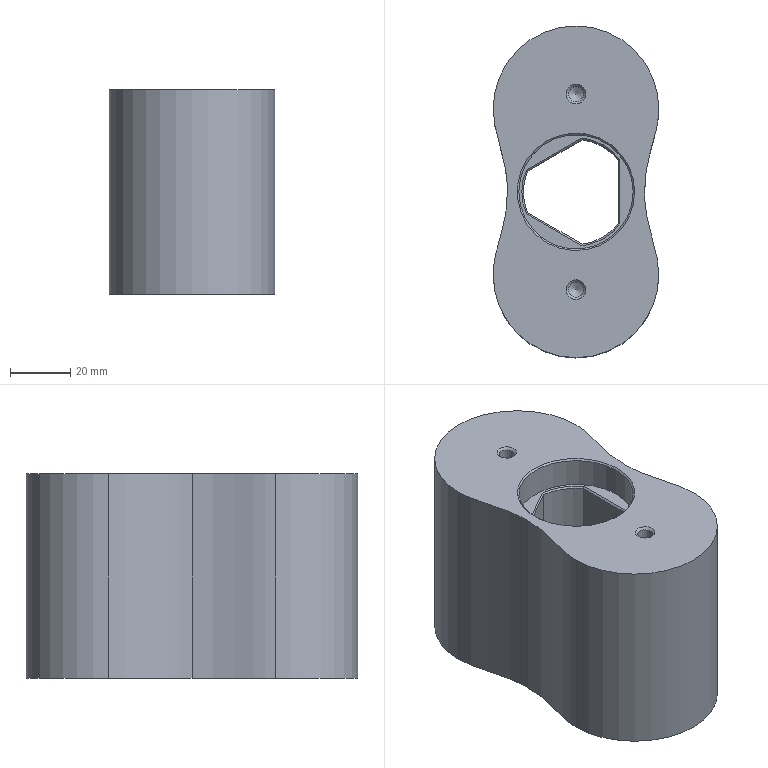NC program | NX | posted with a generic post | part box 55.004 x 110.159 x 68 mm
Lines 1 to 802 of 17802:
N10 G17 G21 G94 G90
(ZLEVEL_PROFILE_COPY , TOOL : D25R0.5)
N12 T05 M6
N14 G54
N16 G17 G0 G90 X42.221 Y-59.812 S2000 M3
N18 G43 Z30. H5
N20 Z-0.349
N22 G94 G1 X40.179 Y-56.265 F1000.
N24 G3 X38.015 Y-55.013 R2.5
N26 G1 X27.71 Y-55.002 F2200.
N28 X26.812 Y-54.988
N30 G2 X14.035 Y-53.354 R57.834
N32 X7.099 Y-51.492 R152.819
N34 G3 X1.947 Y-50.384 R34.294
N36 X-4.924 Y-50.928 R19.124
N38 X-11.562 Y-52.73 R362.576
N40 G2 X-27.952 Y-55.002 R60.697
N42 G1 X-37.557 Y-55.012
N44 G3 X-39.721 Y-56.264 R2.5
N46 G1 X-41.794 Y-59.863
N48 X42.221 Y-59.812 Z-0.697
N50 X40.179 Y-56.265 F1000.
N52 G3 X38.015 Y-55.013 R2.5
N54 G1 X27.71 Y-55.002 F2200.
N56 X26.812 Y-54.988
N58 G2 X14.035 Y-53.354 R57.834
N60 X7.099 Y-51.492 R152.819
N62 G3 X1.947 Y-50.384 R34.294
N64 X-4.924 Y-50.928 R19.124
N66 X-11.562 Y-52.73 R362.576
N68 G2 X-27.952 Y-55.002 R60.697
N70 G1 X-37.557 Y-55.012
N72 G3 X-39.721 Y-56.264 R2.5
N74 G1 X-41.794 Y-59.863
N76 X42.221 Y-59.812 Z-1.046
N78 X40.179 Y-56.265 F1000.
N80 G3 X38.015 Y-55.013 R2.5
N82 G1 X27.71 Y-55.002 F2200.
N84 X26.812 Y-54.988
N86 G2 X14.035 Y-53.354 R57.834
N88 X7.099 Y-51.492 R152.819
N90 G3 X1.947 Y-50.384 R34.294
N92 X-4.924 Y-50.928 R19.124
N94 X-11.562 Y-52.73 R362.576
N96 G2 X-27.952 Y-55.002 R60.697
N98 G1 X-37.557 Y-55.012
N100 G3 X-39.721 Y-56.264 R2.5
N102 G1 X-41.794 Y-59.863
N104 X42.221 Y-59.812 Z-1.395
N106 X40.179 Y-56.265 F1000.
N108 G3 X38.015 Y-55.013 R2.5
N110 G1 X27.71 Y-55.002 F2200.
N112 X26.812 Y-54.988
N114 G2 X14.035 Y-53.354 R57.834
N116 X7.099 Y-51.492 R152.819
N118 G3 X1.947 Y-50.384 R34.294
N120 X-4.924 Y-50.928 R19.124
N122 X-11.562 Y-52.73 R362.576
N124 G2 X-27.952 Y-55.002 R60.697
N126 G1 X-37.557 Y-55.012
N128 G3 X-39.721 Y-56.264 R2.5
N130 G1 X-41.794 Y-59.863
N132 X42.221 Y-59.812 Z-1.744
N134 X40.179 Y-56.265 F1000.
N136 G3 X38.015 Y-55.013 R2.5
N138 G1 X27.71 Y-55.002 F2200.
N140 X26.812 Y-54.988
N142 G2 X14.035 Y-53.354 R57.834
N144 X7.099 Y-51.492 R152.819
N146 G3 X1.947 Y-50.384 R34.294
N148 X-4.924 Y-50.928 R19.124
N150 X-11.562 Y-52.73 R362.576
N152 G2 X-27.952 Y-55.002 R60.697
N154 G1 X-37.557 Y-55.012
N156 G3 X-39.721 Y-56.264 R2.5
N158 G1 X-41.794 Y-59.863
N160 X42.221 Y-59.812 Z-2.092
N162 X40.179 Y-56.265 F1000.
N164 G3 X38.015 Y-55.013 R2.5
N166 G1 X27.71 Y-55.002 F2200.
N168 X26.812 Y-54.988
N170 G2 X14.035 Y-53.354 R57.834
N172 X7.099 Y-51.492 R152.819
N174 G3 X1.947 Y-50.384 R34.294
N176 X-4.924 Y-50.928 R19.124
N178 X-11.562 Y-52.73 R362.576
N180 G2 X-27.952 Y-55.002 R60.697
N182 G1 X-37.557 Y-55.012
N184 G3 X-39.721 Y-56.264 R2.5
N186 G1 X-41.794 Y-59.863
N188 X42.221 Y-59.812 Z-2.441
N190 X40.179 Y-56.265 F1000.
N192 G3 X38.015 Y-55.013 R2.5
N194 G1 X27.71 Y-55.002 F2200.
N196 X26.812 Y-54.988
N198 G2 X14.035 Y-53.354 R57.834
N200 X7.099 Y-51.492 R152.819
N202 G3 X1.947 Y-50.384 R34.294
N204 X-4.924 Y-50.928 R19.124
N206 X-11.562 Y-52.73 R362.576
N208 G2 X-27.952 Y-55.002 R60.697
N210 G1 X-37.557 Y-55.012
N212 G3 X-39.721 Y-56.264 R2.5
N214 G1 X-41.794 Y-59.863
N216 X42.221 Y-59.812 Z-2.79
N218 X40.179 Y-56.265 F1000.
N220 G3 X38.015 Y-55.013 R2.5
N222 G1 X27.71 Y-55.002 F2200.
N224 X26.812 Y-54.988
N226 G2 X14.035 Y-53.354 R57.834
N228 X7.099 Y-51.492 R152.819
N230 G3 X1.947 Y-50.384 R34.294
N232 X-4.924 Y-50.928 R19.124
N234 X-11.562 Y-52.73 R362.576
N236 G2 X-27.952 Y-55.002 R60.698
N238 G1 X-37.557 Y-55.012
N240 G3 X-39.721 Y-56.264 R2.5
N242 G1 X-41.794 Y-59.863
N244 X42.221 Y-59.812 Z-3.138
N246 X40.179 Y-56.265 F1000.
N248 G3 X38.015 Y-55.013 R2.5
N250 G1 X27.71 Y-55.002 F2200.
N252 X26.812 Y-54.988
N254 G2 X14.035 Y-53.354 R57.834
N256 X7.099 Y-51.492 R152.819
N258 G3 X1.947 Y-50.384 R34.294
N260 X-4.924 Y-50.928 R19.124
N262 X-11.562 Y-52.73 R362.576
N264 G2 X-27.952 Y-55.002 R60.698
N266 G1 X-37.557 Y-55.012
N268 G3 X-39.721 Y-56.264 R2.5
N270 G1 X-41.794 Y-59.863
N272 X42.221 Y-59.812 Z-3.487
N274 X40.179 Y-56.265 F1000.
N276 G3 X38.015 Y-55.013 R2.5
N278 G1 X27.71 Y-55.002 F2200.
N280 X26.812 Y-54.988
N282 G2 X14.035 Y-53.354 R57.834
N284 X7.099 Y-51.492 R152.819
N286 G3 X1.947 Y-50.384 R34.294
N288 X-4.924 Y-50.928 R19.124
N290 X-11.562 Y-52.73 R362.576
N292 G2 X-27.952 Y-55.002 R60.698
N294 G1 X-37.557 Y-55.012
N296 G3 X-39.721 Y-56.264 R2.5
N298 G1 X-41.794 Y-59.863
N300 X42.221 Y-59.812 Z-3.836
N302 X40.179 Y-56.265 F1000.
N304 G3 X38.015 Y-55.013 R2.5
N306 G1 X27.71 Y-55.002 F2200.
N308 X26.812 Y-54.988
N310 G2 X14.035 Y-53.354 R57.834
N312 X7.099 Y-51.492 R152.819
N314 G3 X1.947 Y-50.384 R34.294
N316 X-4.924 Y-50.928 R19.124
N318 X-11.562 Y-52.73 R362.576
N320 G2 X-27.952 Y-55.002 R60.698
N322 G1 X-37.557 Y-55.012
N324 G3 X-39.721 Y-56.264 R2.5
N326 G1 X-41.794 Y-59.863
N328 X42.221 Y-59.812 Z-4.185
N330 X40.179 Y-56.265 F1000.
N332 G3 X38.015 Y-55.013 R2.5
N334 G1 X27.71 Y-55.002 F2200.
N336 X26.812 Y-54.988
N338 G2 X14.035 Y-53.354 R57.834
N340 X7.099 Y-51.492 R152.819
N342 G3 X1.947 Y-50.384 R34.294
N344 X-4.924 Y-50.928 R19.124
N346 X-11.562 Y-52.73 R362.576
N348 G2 X-27.952 Y-55.002 R60.698
N350 G1 X-37.557 Y-55.012
N352 G3 X-39.721 Y-56.264 R2.5
N354 G1 X-41.794 Y-59.863
N356 X42.221 Y-59.812 Z-4.533
N358 X40.179 Y-56.265 F1000.
N360 G3 X38.015 Y-55.013 R2.5
N362 G1 X27.71 Y-55.002 F2200.
N364 X26.812 Y-54.988
N366 G2 X14.035 Y-53.354 R57.834
N368 X7.099 Y-51.492 R152.819
N370 G3 X1.947 Y-50.384 R34.294
N372 X-4.924 Y-50.928 R19.124
N374 X-11.562 Y-52.73 R362.576
N376 G2 X-27.952 Y-55.002 R60.698
N378 G1 X-37.557 Y-55.012
N380 G3 X-39.721 Y-56.264 R2.5
N382 G1 X-41.794 Y-59.863
N384 X42.221 Y-59.812 Z-4.882
N386 X40.179 Y-56.265 F1000.
N388 G3 X38.015 Y-55.013 R2.5
N390 G1 X27.71 Y-55.002 F2200.
N392 X26.812 Y-54.988
N394 G2 X14.035 Y-53.354 R57.834
N396 X7.099 Y-51.493 R152.819
N398 G3 X1.947 Y-50.384 R34.294
N400 X-4.924 Y-50.928 R19.124
N402 X-11.562 Y-52.73 R362.576
N404 G2 X-27.952 Y-55.002 R60.698
N406 G1 X-37.557 Y-55.012
N408 G3 X-39.721 Y-56.264 R2.5
N410 G1 X-41.794 Y-59.863
N412 X42.221 Y-59.812 Z-5.231
N414 X40.179 Y-56.265 F1000.
N416 G3 X38.015 Y-55.013 R2.5
N418 G1 X27.71 Y-55.002 F2200.
N420 X26.812 Y-54.988
N422 G2 X14.035 Y-53.354 R57.835
N424 X7.099 Y-51.493 R152.819
N426 G3 X1.947 Y-50.384 R34.294
N428 X-4.924 Y-50.928 R19.124
N430 X-11.562 Y-52.73 R362.576
N432 G2 X-27.952 Y-55.002 R60.698
N434 G1 X-37.557 Y-55.012
N436 G3 X-39.721 Y-56.264 R2.5
N438 G1 X-41.794 Y-59.863
N440 X42.221 Y-59.812 Z-5.579
N442 X40.179 Y-56.265 F1000.
N444 G3 X38.015 Y-55.013 R2.5
N446 G1 X27.71 Y-55.002 F2200.
N448 X26.812 Y-54.988
N450 G2 X14.035 Y-53.354 R57.835
N452 X7.099 Y-51.493 R152.819
N454 G3 X1.947 Y-50.384 R34.294
N456 X-4.924 Y-50.928 R19.124
N458 X-11.562 Y-52.73 R362.576
N460 G2 X-27.952 Y-55.002 R60.698
N462 G1 X-37.557 Y-55.012
N464 G3 X-39.721 Y-56.264 R2.5
N466 G1 X-41.794 Y-59.863
N468 X42.221 Y-59.812 Z-5.928
N470 X40.179 Y-56.265 F1000.
N472 G3 X38.015 Y-55.013 R2.5
N474 G1 X27.71 Y-55.002 F2200.
N476 X26.812 Y-54.988
N478 G2 X14.035 Y-53.354 R57.835
N480 X7.099 Y-51.493 R152.819
N482 G3 X1.947 Y-50.384 R34.294
N484 X-4.924 Y-50.928 R19.124
N486 X-11.562 Y-52.73 R362.576
N488 G2 X-27.952 Y-55.002 R60.698
N490 G1 X-37.557 Y-55.012
N492 G3 X-39.721 Y-56.264 R2.5
N494 G1 X-41.794 Y-59.863
N496 X42.221 Y-59.812 Z-6.277
N498 X40.179 Y-56.265 F1000.
N500 G3 X38.015 Y-55.013 R2.5
N502 G1 X27.71 Y-55.002 F2200.
N504 X26.812 Y-54.988
N506 G2 X14.035 Y-53.354 R57.835
N508 X7.099 Y-51.493 R152.819
N510 G3 X1.947 Y-50.384 R34.294
N512 X-4.924 Y-50.928 R19.124
N514 X-11.562 Y-52.73 R362.576
N516 G2 X-27.952 Y-55.002 R60.698
N518 G1 X-37.557 Y-55.012
N520 G3 X-39.721 Y-56.264 R2.5
N522 G1 X-41.794 Y-59.863
N524 X42.221 Y-59.812 Z-6.626
N526 X40.179 Y-56.265 F1000.
N528 G3 X38.015 Y-55.013 R2.5
N530 G1 X27.71 Y-55.002 F2200.
N532 X26.812 Y-54.988
N534 G2 X14.035 Y-53.354 R57.835
N536 X7.099 Y-51.493 R152.819
N538 G3 X1.947 Y-50.384 R34.294
N540 X-4.924 Y-50.928 R19.124
N542 X-11.562 Y-52.73 R362.576
N544 G2 X-27.952 Y-55.002 R60.699
N546 G1 X-37.557 Y-55.012
N548 G3 X-39.721 Y-56.264 R2.5
N550 G1 X-41.794 Y-59.863
N552 X42.221 Y-59.812 Z-6.974
N554 X40.179 Y-56.265 F1000.
N556 G3 X38.015 Y-55.013 R2.5
N558 G1 X27.71 Y-55.002 F2200.
N560 X26.812 Y-54.988
N562 G2 X14.035 Y-53.354 R57.835
N564 X7.099 Y-51.493 R152.819
N566 G3 X1.947 Y-50.384 R34.294
N568 X-4.924 Y-50.928 R19.124
N570 X-11.562 Y-52.73 R362.576
N572 G2 X-27.952 Y-55.002 R60.699
N574 G1 X-37.557 Y-55.012
N576 G3 X-39.721 Y-56.264 R2.5
N578 G1 X-41.794 Y-59.863
N580 X42.221 Y-59.812 Z-7.323
N582 X40.179 Y-56.265 F1000.
N584 G3 X38.015 Y-55.013 R2.5
N586 G1 X27.71 Y-55.002 F2200.
N588 X26.812 Y-54.988
N590 G2 X14.035 Y-53.354 R57.835
N592 X7.099 Y-51.493 R152.819
N594 G3 X1.947 Y-50.384 R34.294
N596 X-4.924 Y-50.928 R19.124
N598 X-11.562 Y-52.73 R362.576
N600 G2 X-27.952 Y-55.002 R60.699
N602 G1 X-37.557 Y-55.012
N604 G3 X-39.721 Y-56.264 R2.5
N606 G1 X-41.794 Y-59.863
N608 X42.221 Y-59.812 Z-7.672
N610 X40.179 Y-56.265 F1000.
N612 G3 X38.015 Y-55.013 R2.5
N614 G1 X27.71 Y-55.002 F2200.
N616 X26.812 Y-54.988
N618 G2 X14.035 Y-53.354 R57.835
N620 X7.099 Y-51.493 R152.819
N622 G3 X1.947 Y-50.384 R34.294
N624 X-4.924 Y-50.928 R19.124
N626 X-11.561 Y-52.73 R362.576
N628 G2 X-27.952 Y-55.002 R60.699
N630 G1 X-37.557 Y-55.012
N632 G3 X-39.721 Y-56.264 R2.5
N634 G1 X-41.794 Y-59.863
N636 X42.221 Y-59.812 Z-8.021
N638 X40.179 Y-56.265 F1000.
N640 G3 X38.015 Y-55.013 R2.5
N642 G1 X27.71 Y-55.002 F2200.
N644 X26.812 Y-54.988
N646 G2 X14.035 Y-53.354 R57.835
N648 X7.099 Y-51.493 R152.819
N650 G3 X1.947 Y-50.384 R34.294
N652 X-4.924 Y-50.928 R19.124
N654 X-11.561 Y-52.73 R362.576
N656 G2 X-27.952 Y-55.002 R60.699
N658 G1 X-37.557 Y-55.012
N660 G3 X-39.721 Y-56.264 R2.5
N662 G1 X-41.794 Y-59.863
N664 X42.221 Y-59.812 Z-8.369
N666 X40.179 Y-56.265 F1000.
N668 G3 X38.015 Y-55.013 R2.5
N670 G1 X27.71 Y-55.002 F2200.
N672 X26.812 Y-54.988
N674 G2 X14.035 Y-53.354 R57.835
N676 X7.099 Y-51.493 R152.819
N678 G3 X1.947 Y-50.384 R34.294
N680 X-4.924 Y-50.928 R19.124
N682 X-11.561 Y-52.73 R362.576
N684 G2 X-27.952 Y-55.002 R60.699
N686 G1 X-37.557 Y-55.012
N688 G3 X-39.721 Y-56.264 R2.5
N690 G1 X-41.794 Y-59.863
N692 X42.221 Y-59.812 Z-8.718
N694 X40.179 Y-56.265 F1000.
N696 G3 X38.015 Y-55.013 R2.5
N698 G1 X27.71 Y-55.002 F2200.
N700 X26.812 Y-54.988
N702 G2 X14.035 Y-53.354 R57.835
N704 X7.099 Y-51.493 R152.819
N706 G3 X1.947 Y-50.384 R34.294
N708 X-4.924 Y-50.928 R19.124
N710 X-11.561 Y-52.73 R362.576
N712 G2 X-27.952 Y-55.002 R60.699
N714 G1 X-37.557 Y-55.012
N716 G3 X-39.721 Y-56.264 R2.5
N718 G1 X-41.794 Y-59.863
N720 X42.221 Y-59.812 Z-9.067
N722 X40.179 Y-56.265 F1000.
N724 G3 X38.015 Y-55.013 R2.5
N726 G1 X27.71 Y-55.002 F2200.
N728 X26.812 Y-54.988
N730 G2 X14.035 Y-53.354 R57.835
N732 X7.099 Y-51.493 R152.819
N734 G3 X1.947 Y-50.384 R34.294
N736 X-4.924 Y-50.928 R19.124
N738 X-11.561 Y-52.73 R362.576
N740 G2 X-27.952 Y-55.002 R60.699
N742 G1 X-37.557 Y-55.012
N744 G3 X-39.721 Y-56.264 R2.5
N746 G1 X-41.794 Y-59.863
N748 X42.221 Y-59.812 Z-9.415
N750 X40.179 Y-56.265 F1000.
N752 G3 X38.015 Y-55.013 R2.5
N754 G1 X27.71 Y-55.002 F2200.
N756 X26.812 Y-54.988
N758 G2 X14.035 Y-53.354 R57.835
N760 X7.099 Y-51.493 R152.819
N762 G3 X1.947 Y-50.384 R34.294
N764 X-4.924 Y-50.928 R19.124
N766 X-11.561 Y-52.73 R362.576
N768 G2 X-27.952 Y-55.002 R60.699
N770 G1 X-37.557 Y-55.012
N772 G3 X-39.721 Y-56.264 R2.5
N774 G1 X-41.794 Y-59.863
N776 X42.221 Y-59.812 Z-9.764
N778 X40.179 Y-56.265 F1000.
N780 G3 X38.015 Y-55.013 R2.5
N782 G1 X27.71 Y-55.002 F2200.
N784 X26.812 Y-54.988
N786 G2 X14.035 Y-53.354 R57.835
N788 X7.099 Y-51.493 R152.819
N790 G3 X1.947 Y-50.384 R34.294
N792 X-4.924 Y-50.928 R19.124
N794 X-11.561 Y-52.73 R362.576
N796 G2 X-27.952 Y-55.002 R60.699
N798 G1 X-37.557 Y-55.012
N800 G3 X-39.721 Y-56.264 R2.5
N802 G1 X-41.794 Y-59.863
N804 X42.221 Y-59.812 Z-10.113
N806 X40.179 Y-56.265 F1000.
N808 G3 X38.015 Y-55.013 R2.5
N810 G1 X27.71 Y-55.002 F2200.
N812 X26.812 Y-54.988
N814 G2 X14.035 Y-53.354 R57.836
N816 X7.099 Y-51.493 R152.819
N818 G3 X1.947 Y-50.384 R34.294
N820 X-4.924 Y-50.928 R19.124
N822 X-11.561 Y-52.73 R362.576
N824 G2 X-27.952 Y-55.002 R60.7
N826 G1 X-37.557 Y-55.012
N828 G3 X-39.721 Y-56.264 R2.5
N830 G1 X-41.794 Y-59.863
N832 X42.221 Y-59.812 Z-10.462
N834 X40.179 Y-56.265 F1000.
N836 G3 X38.015 Y-55.013 R2.5
N838 G1 X27.71 Y-55.002 F2200.
N840 X26.812 Y-54.988
N842 G2 X14.035 Y-53.354 R57.836
N844 X7.099 Y-51.493 R152.819
N846 G3 X1.947 Y-50.384 R34.294
N848 X-4.924 Y-50.928 R19.124
N850 X-11.561 Y-52.73 R362.576
N852 G2 X-27.952 Y-55.002 R60.7
N854 G1 X-37.557 Y-55.012
N856 G3 X-39.721 Y-56.264 R2.5
N858 G1 X-41.794 Y-59.863
N860 X42.221 Y-59.812 Z-10.81
N862 X40.179 Y-56.265 F1000.
N864 G3 X38.015 Y-55.013 R2.5
N866 G1 X27.71 Y-55.002 F2200.
N868 X26.812 Y-54.988
N870 G2 X14.035 Y-53.354 R57.836
N872 X7.099 Y-51.493 R152.819
N874 G3 X1.947 Y-50.384 R34.294
N876 X-4.924 Y-50.928 R19.124
N878 X-11.561 Y-52.73 R362.576
N880 G2 X-27.952 Y-55.002 R60.7
N882 G1 X-37.557 Y-55.012
N884 G3 X-39.721 Y-56.264 R2.5
N886 G1 X-41.794 Y-59.863
N888 X42.221 Y-59.812 Z-11.159
N890 X40.179 Y-56.265 F1000.
N892 G3 X38.015 Y-55.013 R2.5
N894 G1 X27.71 Y-55.002 F2200.
N896 X26.812 Y-54.988
N898 G2 X14.034 Y-53.354 R57.836
N900 X7.099 Y-51.493 R152.819
N902 G3 X1.947 Y-50.384 R34.294
N904 X-4.924 Y-50.928 R19.124
N906 X-11.561 Y-52.73 R362.576
N908 G2 X-27.952 Y-55.002 R60.7
N910 G1 X-37.557 Y-55.012
N912 G3 X-39.721 Y-56.264 R2.5
N914 G1 X-41.794 Y-59.863
N916 X42.221 Y-59.812 Z-11.508
N918 X40.179 Y-56.265 F1000.
N920 G3 X38.015 Y-55.013 R2.5
N922 G1 X27.71 Y-55.002 F2200.
N924 X26.812 Y-54.988
N926 G2 X14.034 Y-53.354 R57.836
N928 X7.099 Y-51.493 R152.819
N930 G3 X1.947 Y-50.384 R34.294
N932 X-4.924 Y-50.928 R19.124
N934 X-11.561 Y-52.73 R362.576
N936 G2 X-27.952 Y-55.002 R60.7
N938 G1 X-37.557 Y-55.012
N940 G3 X-39.721 Y-56.264 R2.5
N942 G1 X-41.794 Y-59.863
N944 X42.221 Y-59.812 Z-11.856
N946 X40.179 Y-56.265 F1000.
N948 G3 X38.015 Y-55.013 R2.5
N950 G1 X27.71 Y-55.002 F2200.
N952 X26.812 Y-54.988
N954 G2 X14.034 Y-53.354 R57.836
N956 X7.099 Y-51.493 R152.819
N958 G3 X1.947 Y-50.384 R34.294
N960 X-4.924 Y-50.928 R19.124
N962 X-11.561 Y-52.73 R362.576
N964 G2 X-27.952 Y-55.002 R60.7
N966 G1 X-37.557 Y-55.012
N968 G3 X-39.721 Y-56.264 R2.5
N970 G1 X-41.794 Y-59.863
N972 X42.221 Y-59.812 Z-12.205
N974 X40.179 Y-56.265 F1000.
N976 G3 X38.015 Y-55.013 R2.5
N978 G1 X27.71 Y-55.002 F2200.
N980 X26.812 Y-54.988
N982 G2 X14.034 Y-53.354 R57.836
N984 X7.099 Y-51.493 R152.819
N986 G3 X1.947 Y-50.384 R34.294
N988 X-4.924 Y-50.928 R19.124
N990 X-11.561 Y-52.73 R362.576
N992 G2 X-27.952 Y-55.002 R60.7
N994 G1 X-37.557 Y-55.012
N996 G3 X-39.721 Y-56.264 R2.5
N998 G1 X-41.794 Y-59.863
N1000 X42.221 Y-59.812 Z-12.554
N1002 X40.179 Y-56.265 F1000.
N1004 G3 X38.015 Y-55.013 R2.5
N1006 G1 X27.71 Y-55.002 F2200.
N1008 X26.812 Y-54.988
N1010 G2 X14.034 Y-53.354 R57.836
N1012 X7.099 Y-51.493 R152.819
N1014 G3 X1.947 Y-50.384 R34.294
N1016 X-4.924 Y-50.928 R19.124
N1018 X-11.561 Y-52.73 R362.576
N1020 G2 X-27.952 Y-55.002 R60.7
N1022 G1 X-37.557 Y-55.012
N1024 G3 X-39.721 Y-56.264 R2.5
N1026 G1 X-41.794 Y-59.863
N1028 X42.221 Y-59.812 Z-12.903
N1030 X40.179 Y-56.265 F1000.
N1032 G3 X38.015 Y-55.013 R2.5
N1034 G1 X27.71 Y-55.002 F2200.
N1036 X26.812 Y-54.988
N1038 G2 X14.034 Y-53.354 R57.836
N1040 X7.099 Y-51.493 R152.819
N1042 G3 X1.947 Y-50.384 R34.294
N1044 X-4.924 Y-50.928 R19.124
N1046 X-11.561 Y-52.73 R362.576
N1048 G2 X-27.952 Y-55.002 R60.7
N1050 G1 X-37.557 Y-55.012
N1052 G3 X-39.721 Y-56.264 R2.5
N1054 G1 X-41.794 Y-59.863
N1056 X42.221 Y-59.812 Z-13.251
N1058 X40.179 Y-56.265 F1000.
N1060 G3 X38.015 Y-55.013 R2.5
N1062 G1 X27.71 Y-55.002 F2200.
N1064 X26.812 Y-54.988
N1066 G2 X14.034 Y-53.354 R57.836
N1068 X7.099 Y-51.493 R152.819
N1070 G3 X1.947 Y-50.384 R34.294
N1072 X-4.924 Y-50.928 R19.124
N1074 X-11.561 Y-52.73 R362.576
N1076 G2 X-27.952 Y-55.002 R60.7
N1078 G1 X-37.557 Y-55.012
N1080 G3 X-39.721 Y-56.264 R2.5
N1082 G1 X-41.794 Y-59.863
N1084 X42.221 Y-59.812 Z-13.6
N1086 X40.179 Y-56.265 F1000.
N1088 G3 X38.015 Y-55.013 R2.5
N1090 G1 X27.71 Y-55.002 F2200.
N1092 X26.812 Y-54.988
N1094 G2 X14.034 Y-53.354 R57.836
N1096 X7.099 Y-51.493 R152.819
N1098 G3 X1.947 Y-50.384 R34.294
N1100 X-4.924 Y-50.928 R19.124
N1102 X-11.561 Y-52.73 R362.576
N1104 G2 X-27.953 Y-55.002 R60.701
N1106 G1 X-37.557 Y-55.012
N1108 G3 X-39.721 Y-56.264 R2.5
N1110 G1 X-41.794 Y-59.863
N1112 X42.221 Y-59.812 Z-13.949
N1114 X40.179 Y-56.265 F1000.
N1116 G3 X38.015 Y-55.013 R2.5
N1118 G1 X27.71 Y-55.002 F2200.
N1120 X26.812 Y-54.988
N1122 G2 X14.034 Y-53.354 R57.836
N1124 X7.099 Y-51.493 R152.819
N1126 G3 X1.947 Y-50.384 R34.294
N1128 X-4.924 Y-50.928 R19.124
N1130 X-11.561 Y-52.73 R362.576
N1132 G2 X-27.953 Y-55.002 R60.701
N1134 G1 X-37.557 Y-55.012
N1136 G3 X-39.721 Y-56.264 R2.5
N1138 G1 X-41.794 Y-59.863
N1140 X42.221 Y-59.812 Z-14.297
N1142 X40.179 Y-56.265 F1000.
N1144 G3 X38.015 Y-55.013 R2.5
N1146 G1 X27.71 Y-55.002 F2200.
N1148 X26.812 Y-54.988
N1150 G2 X14.034 Y-53.354 R57.836
N1152 X7.099 Y-51.493 R152.819
N1154 G3 X1.947 Y-50.384 R34.294
N1156 X-4.924 Y-50.928 R19.124
N1158 X-11.561 Y-52.73 R362.576
N1160 G2 X-27.953 Y-55.002 R60.701
N1162 G1 X-37.557 Y-55.012
N1164 G3 X-39.721 Y-56.264 R2.5
N1166 G1 X-41.794 Y-59.863
N1168 X42.221 Y-59.812 Z-14.646
N1170 X40.179 Y-56.265 F1000.
N1172 G3 X38.015 Y-55.013 R2.5
N1174 G1 X27.71 Y-55.002 F2200.
N1176 X26.812 Y-54.988
N1178 G2 X14.034 Y-53.354 R57.836
N1180 X7.099 Y-51.493 R152.819
N1182 G3 X1.947 Y-50.384 R34.294
N1184 X-4.924 Y-50.928 R19.124
N1186 X-11.561 Y-52.73 R362.576
N1188 G2 X-27.953 Y-55.002 R60.701
N1190 G1 X-37.557 Y-55.012
N1192 G3 X-39.721 Y-56.264 R2.5
N1194 G1 X-41.794 Y-59.863
N1196 X42.221 Y-59.812 Z-14.995
N1198 X40.179 Y-56.265 F1000.
N1200 G3 X38.015 Y-55.013 R2.5
N1202 G1 X27.71 Y-55.002 F2200.
N1204 X26.812 Y-54.988
N1206 G2 X14.034 Y-53.354 R57.837
N1208 X7.099 Y-51.493 R152.819
N1210 G3 X1.947 Y-50.384 R34.294
N1212 X-4.924 Y-50.928 R19.124
N1214 X-11.561 Y-52.73 R362.576
N1216 G2 X-27.953 Y-55.002 R60.701
N1218 G1 X-37.557 Y-55.012
N1220 G3 X-39.721 Y-56.264 R2.5
N1222 G1 X-41.794 Y-59.863
N1224 X42.221 Y-59.812 Z-15.344
N1226 X40.179 Y-56.265 F1000.
N1228 G3 X38.015 Y-55.013 R2.5
N1230 G1 X27.71 Y-55.002 F2200.
N1232 X26.812 Y-54.988
N1234 G2 X14.034 Y-53.354 R57.837
N1236 X7.099 Y-51.493 R152.819
N1238 G3 X1.947 Y-50.384 R34.294
N1240 X-4.924 Y-50.928 R19.124
N1242 X-11.561 Y-52.73 R362.576
N1244 G2 X-27.953 Y-55.002 R60.701
N1246 G1 X-37.557 Y-55.012
N1248 G3 X-39.721 Y-56.264 R2.5
N1250 G1 X-41.794 Y-59.863
N1252 X42.221 Y-59.812 Z-15.692
N1254 X40.179 Y-56.265 F1000.
N1256 G3 X38.015 Y-55.013 R2.5
N1258 G1 X27.71 Y-55.002 F2200.
N1260 X26.812 Y-54.988
N1262 G2 X14.034 Y-53.354 R57.837
N1264 X7.099 Y-51.493 R152.819
N1266 G3 X1.947 Y-50.384 R34.294
N1268 X-4.924 Y-50.928 R19.124
N1270 X-11.561 Y-52.73 R362.576
N1272 G2 X-27.953 Y-55.002 R60.701
N1274 G1 X-37.557 Y-55.012
N1276 G3 X-39.721 Y-56.264 R2.5
N1278 G1 X-41.794 Y-59.863
N1280 X42.221 Y-59.812 Z-16.041
N1282 X40.179 Y-56.265 F1000.
N1284 G3 X38.015 Y-55.013 R2.5
N1286 G1 X27.71 Y-55.002 F2200.
N1288 X26.811 Y-54.988
N1290 G2 X14.034 Y-53.354 R57.837
N1292 X7.099 Y-51.493 R152.819
N1294 G3 X1.947 Y-50.384 R34.294
N1296 X-4.924 Y-50.928 R19.124
N1298 X-11.561 Y-52.73 R362.576
N1300 G2 X-27.953 Y-55.002 R60.701
N1302 G1 X-37.557 Y-55.012
N1304 G3 X-39.721 Y-56.264 R2.5
N1306 G1 X-41.794 Y-59.863
N1308 X42.221 Y-59.812 Z-16.39
N1310 X40.179 Y-56.265 F1000.
N1312 G3 X38.015 Y-55.013 R2.5
N1314 G1 X27.71 Y-55.002 F2200.
N1316 X26.811 Y-54.988
N1318 G2 X14.034 Y-53.354 R57.837
N1320 X7.099 Y-51.493 R152.819
N1322 G3 X1.947 Y-50.384 R34.294
N1324 X-4.924 Y-50.928 R19.124
N1326 X-11.561 Y-52.73 R362.576
N1328 G2 X-27.953 Y-55.002 R60.701
N1330 G1 X-37.557 Y-55.012
N1332 G3 X-39.721 Y-56.264 R2.5
N1334 G1 X-41.794 Y-59.863
N1336 X42.221 Y-59.812 Z-16.738
N1338 X40.179 Y-56.265 F1000.
N1340 G3 X38.015 Y-55.013 R2.5
N1342 G1 X27.71 Y-55.002 F2200.
N1344 X26.811 Y-54.988
N1346 G2 X14.034 Y-53.354 R57.837
N1348 X7.099 Y-51.493 R152.819
N1350 G3 X1.947 Y-50.384 R34.294
N1352 X-4.924 Y-50.928 R19.124
N1354 X-11.561 Y-52.73 R362.576
N1356 G2 X-27.953 Y-55.002 R60.701
N1358 G1 X-37.557 Y-55.012
N1360 G3 X-39.721 Y-56.264 R2.5
N1362 G1 X-41.794 Y-59.863
N1364 X42.221 Y-59.812 Z-17.087
N1366 X40.179 Y-56.265 F1000.
N1368 G3 X38.015 Y-55.013 R2.5
N1370 G1 X27.71 Y-55.002 F2200.
N1372 X26.811 Y-54.988
N1374 G2 X14.034 Y-53.354 R57.837
N1376 X7.099 Y-51.493 R152.819
N1378 G3 X1.947 Y-50.384 R34.294
N1380 X-4.924 Y-50.928 R19.124
N1382 X-11.561 Y-52.73 R362.576
N1384 G2 X-27.953 Y-55.002 R60.701
N1386 G1 X-37.557 Y-55.012
N1388 G3 X-39.721 Y-56.264 R2.5
N1390 G1 X-41.794 Y-59.863
N1392 X42.221 Y-59.812 Z-17.436
N1394 X40.179 Y-56.265 F1000.
N1396 G3 X38.015 Y-55.013 R2.5
N1398 G1 X27.71 Y-55.002 F2200.
N1400 X26.811 Y-54.988
N1402 G2 X14.034 Y-53.354 R57.837
N1404 X7.099 Y-51.493 R152.819
N1406 G3 X1.947 Y-50.384 R34.294
N1408 X-4.924 Y-50.928 R19.124
N1410 X-11.561 Y-52.73 R362.576
N1412 G2 X-27.953 Y-55.002 R60.702
N1414 G1 X-37.557 Y-55.012
N1416 G3 X-39.721 Y-56.264 R2.5
N1418 G1 X-41.794 Y-59.863
N1420 X42.221 Y-59.812 Z-17.785
N1422 X40.179 Y-56.265 F1000.
N1424 G3 X38.015 Y-55.013 R2.5
N1426 G1 X27.71 Y-55.002 F2200.
N1428 X26.811 Y-54.988
N1430 G2 X14.034 Y-53.354 R57.837
N1432 X7.099 Y-51.493 R152.819
N1434 G3 X1.947 Y-50.384 R34.294
N1436 X-4.924 Y-50.928 R19.124
N1438 X-11.561 Y-52.73 R362.576
N1440 G2 X-27.953 Y-55.002 R60.702
N1442 G1 X-37.557 Y-55.012
N1444 G3 X-39.721 Y-56.264 R2.5
N1446 G1 X-41.794 Y-59.863
N1448 X42.221 Y-59.812 Z-18.133
N1450 X40.179 Y-56.265 F1000.
N1452 G3 X38.015 Y-55.013 R2.5
N1454 G1 X27.71 Y-55.002 F2200.
N1456 X26.811 Y-54.988
N1458 G2 X14.034 Y-53.354 R57.837
N1460 X7.099 Y-51.493 R152.819
N1462 G3 X1.947 Y-50.384 R34.294
N1464 X-4.924 Y-50.928 R19.124
N1466 X-11.561 Y-52.73 R362.576
N1468 G2 X-27.953 Y-55.002 R60.702
N1470 G1 X-37.557 Y-55.012
N1472 G3 X-39.721 Y-56.264 R2.5
N1474 G1 X-41.794 Y-59.863
N1476 X42.221 Y-59.812 Z-18.482
N1478 X40.179 Y-56.265 F1000.
N1480 G3 X38.015 Y-55.013 R2.5
N1482 G1 X27.71 Y-55.002 F2200.
N1484 X26.811 Y-54.988
N1486 G2 X14.034 Y-53.354 R57.837
N1488 X7.099 Y-51.493 R152.819
N1490 G3 X1.947 Y-50.384 R34.294
N1492 X-4.924 Y-50.928 R19.124
N1494 X-11.561 Y-52.73 R362.576
N1496 G2 X-27.953 Y-55.002 R60.702
N1498 G1 X-37.557 Y-55.012
N1500 G3 X-39.721 Y-56.264 R2.5
N1502 G1 X-41.794 Y-59.863
N1504 X42.221 Y-59.812 Z-18.831
N1506 X40.179 Y-56.265 F1000.
N1508 G3 X38.015 Y-55.013 R2.5
N1510 G1 X27.71 Y-55.002 F2200.
N1512 X26.811 Y-54.988
N1514 G2 X14.034 Y-53.354 R57.837
N1516 X7.099 Y-51.493 R152.819
N1518 G3 X1.947 Y-50.384 R34.294
N1520 X-4.924 Y-50.928 R19.124
N1522 X-11.561 Y-52.73 R362.576
N1524 G2 X-27.953 Y-55.002 R60.702
N1526 G1 X-37.557 Y-55.012
N1528 G3 X-39.721 Y-56.264 R2.5
N1530 G1 X-41.794 Y-59.863
N1532 X42.221 Y-59.812 Z-19.179
N1534 X40.179 Y-56.265 F1000.
N1536 G3 X38.015 Y-55.013 R2.5
N1538 G1 X27.71 Y-55.002 F2200.
N1540 X26.811 Y-54.988
N1542 G2 X14.034 Y-53.354 R57.837
N1544 X7.099 Y-51.493 R152.819
N1546 G3 X1.947 Y-50.384 R34.294
N1548 X-4.924 Y-50.928 R19.124
N1550 X-11.561 Y-52.73 R362.576
N1552 G2 X-27.953 Y-55.002 R60.702
N1554 G1 X-37.557 Y-55.012
N1556 G3 X-39.721 Y-56.264 R2.5
N1558 G1 X-41.794 Y-59.863
N1560 X42.221 Y-59.812 Z-19.528
N1562 X40.179 Y-56.265 F1000.
N1564 G3 X38.015 Y-55.013 R2.5
N1566 G1 X27.71 Y-55.002 F2200.
N1568 X26.811 Y-54.988
N1570 G2 X14.034 Y-53.354 R57.837
N1572 X7.099 Y-51.493 R152.819
N1574 G3 X1.947 Y-50.384 R34.294
N1576 X-4.924 Y-50.928 R19.124
N1578 X-11.561 Y-52.73 R362.576
N1580 G2 X-27.953 Y-55.002 R60.702
N1582 G1 X-37.557 Y-55.012
N1584 G3 X-39.721 Y-56.264 R2.5
N1586 G1 X-41.794 Y-59.863
N1588 X42.221 Y-59.812 Z-19.877
N1590 X40.179 Y-56.265 F1000.
N1592 G3 X38.015 Y-55.013 R2.5
N1594 G1 X27.71 Y-55.002 F2200.
N1596 X26.811 Y-54.988
N1598 G2 X14.034 Y-53.354 R57.838
N1600 X7.099 Y-51.493 R152.819
N1602 G3 X1.947 Y-50.384 R34.294